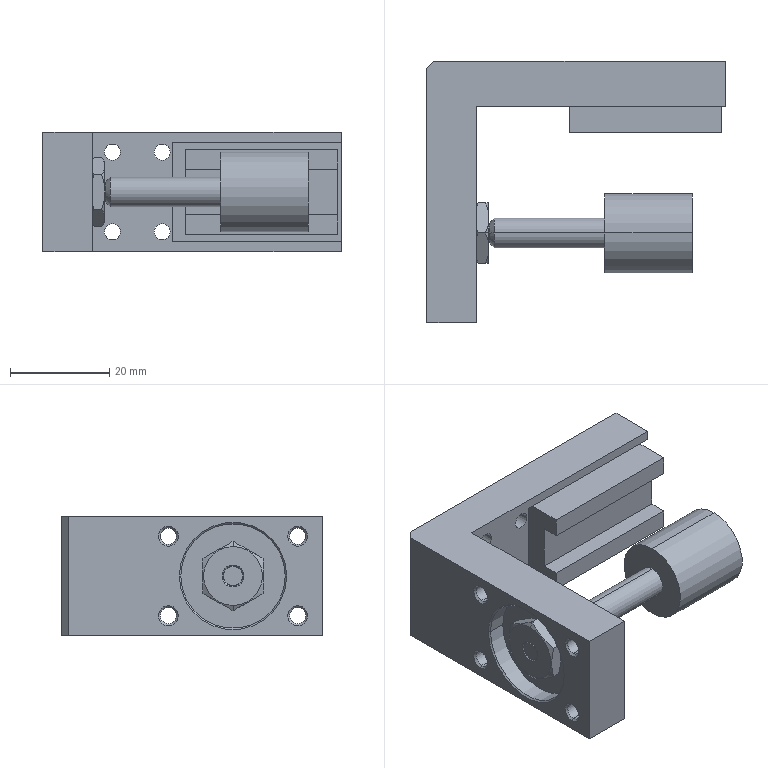Part | SolidWorks | features BaseBody 1 | 1 solid | 167 faces | box 60 x 52.5 x 24 mm | volume 27442 mm3 | cone 60 | plane 51 | cylinder 48 | spline 8 | commonest cylinder face diameters 3.242 x16 6 x10 2.88 x8 5.5 x8 4 x2 16 x2